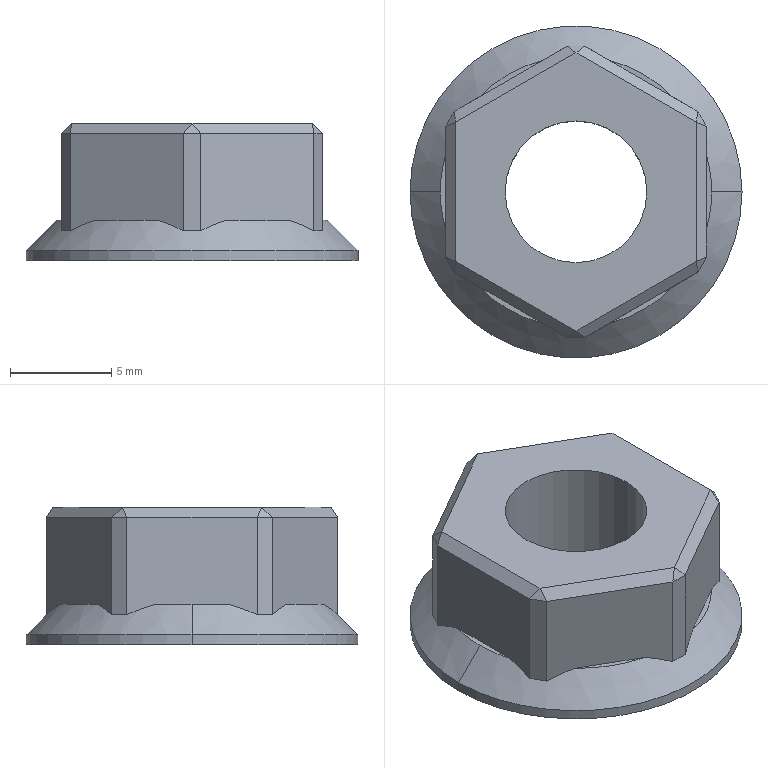Part | SolidWorks | features BaseBody 1 | 1 solid | 38 faces | box 16.4 x 16.4 x 6.8 mm | volume 790.992 mm3 | plane 32 | cylinder 4 | cone 2 | commonest cylinder face diameters 7 x2 16.4 x2
STEP:
#1=CARTESIAN_POINT('',(-8.2,0.,0.5));
#2=VERTEX_POINT('',#1);
#3=CARTESIAN_POINT('',(8.2,0.,0.5));
#4=VERTEX_POINT('',#3);
#5=CARTESIAN_POINT('',(0.,0.,0.5));
#6=DIRECTION('',(0.,0.,-1.));
#7=DIRECTION('',(-1.,0.,0.));
#8=AXIS2_PLACEMENT_3D('',#5,#6,#7);
#9=CIRCLE('',#8,8.2);
#10=EDGE_CURVE('',#2,#4,#9,.T.);
#11=ORIENTED_EDGE('',*,*,#10,.T.);
#12=CARTESIAN_POINT('',(8.2,0.,0.));
#13=VERTEX_POINT('',#12);
#14=CARTESIAN_POINT('',(8.2,0.,2.));
#15=DIRECTION('',(0.,0.,-1.));
#16=VECTOR('',#15,1000.);
#17=LINE('',#14,#16);
#18=EDGE_CURVE('',#4,#13,#17,.T.);
#19=ORIENTED_EDGE('',*,*,#18,.T.);
#20=CARTESIAN_POINT('',(-8.2,0.,0.));
#21=VERTEX_POINT('',#20);
#22=CARTESIAN_POINT('',(0.,0.,0.));
#23=DIRECTION('',(0.,0.,1.));
#24=DIRECTION('',(-1.,0.,0.));
#25=AXIS2_PLACEMENT_3D('',#22,#23,#24);
#26=CIRCLE('',#25,8.2);
#27=EDGE_CURVE('',#13,#21,#26,.T.);
#28=ORIENTED_EDGE('',*,*,#27,.T.);
#29=CARTESIAN_POINT('',(-8.2,0.,2.));
#30=DIRECTION('',(0.,0.,-1.));
#31=VECTOR('',#30,1000.);
#32=LINE('',#29,#31);
#33=EDGE_CURVE('',#2,#21,#32,.T.);
#34=ORIENTED_EDGE('',*,*,#33,.F.);
#35=EDGE_LOOP('',(#11,#19,#28,#34));
#36=FACE_OUTER_BOUND('',#35,.T.);
#37=CARTESIAN_POINT('',(0.,0.,2.));
#38=DIRECTION('',(0.,0.,-1.));
#39=DIRECTION('',(-1.,0.,0.));
#40=AXIS2_PLACEMENT_3D('',#37,#38,#39);
#41=CYLINDRICAL_SURFACE('',#40,8.2);
#42=ADVANCED_FACE('',(#36),#41,.T.);
#43=CARTESIAN_POINT('',(3.5,0.,0.));
#44=VERTEX_POINT('',#43);
#45=CARTESIAN_POINT('',(-3.5,0.,0.));
#46=VERTEX_POINT('',#45);
#47=CARTESIAN_POINT('',(0.,0.,0.));
#48=DIRECTION('',(0.,0.,-1.));
#49=DIRECTION('',(1.,0.,0.));
#50=AXIS2_PLACEMENT_3D('',#47,#48,#49);
#51=CIRCLE('',#50,3.5);
#52=EDGE_CURVE('',#44,#46,#51,.T.);
#53=ORIENTED_EDGE('',*,*,#52,.T.);
#54=CARTESIAN_POINT('',(-3.5,0.,6.8));
#55=VERTEX_POINT('',#54);
#56=CARTESIAN_POINT('',(-3.5,0.,6.8));
#57=DIRECTION('',(0.,0.,1.));
#58=VECTOR('',#57,1000.);
#59=LINE('',#56,#58);
#60=EDGE_CURVE('',#46,#55,#59,.T.);
#61=ORIENTED_EDGE('',*,*,#60,.T.);
#62=CARTESIAN_POINT('',(3.5,0.,6.8));
#63=VERTEX_POINT('',#62);
#64=CARTESIAN_POINT('',(0.,0.,6.8));
#65=DIRECTION('',(0.,0.,-1.));
#66=DIRECTION('',(1.,0.,0.));
#67=AXIS2_PLACEMENT_3D('',#64,#65,#66);
#68=CIRCLE('',#67,3.5);
#69=EDGE_CURVE('',#63,#55,#68,.T.);
#70=ORIENTED_EDGE('',*,*,#69,.F.);
#71=CARTESIAN_POINT('',(3.5,0.,6.8));
#72=DIRECTION('',(0.,0.,1.));
#73=VECTOR('',#72,1000.);
#74=LINE('',#71,#73);
#75=EDGE_CURVE('',#44,#63,#74,.T.);
#76=ORIENTED_EDGE('',*,*,#75,.F.);
#77=EDGE_LOOP('',(#53,#61,#70,#76));
#78=FACE_OUTER_BOUND('',#77,.T.);
#79=CARTESIAN_POINT('',(0.,0.,6.8));
#80=DIRECTION('',(0.,0.,1.));
#81=DIRECTION('',(1.,0.,0.));
#82=AXIS2_PLACEMENT_3D('',#79,#80,#81);
#83=CYLINDRICAL_SURFACE('',#82,3.5);
#84=ADVANCED_FACE('',(#78),#83,.F.);
#85=CARTESIAN_POINT('',(6.45,1.813,2.));
#86=VERTEX_POINT('',#85);
#87=CARTESIAN_POINT('',(6.7,0.,2.));
#88=VERTEX_POINT('',#87);
#89=CARTESIAN_POINT('',(0.,0.,2.));
#90=DIRECTION('',(0.,0.,-1.));
#91=DIRECTION('',(-1.,0.,0.));
#92=AXIS2_PLACEMENT_3D('',#89,#90,#91);
#93=CIRCLE('',#92,6.7);
#94=EDGE_CURVE('',#86,#88,#93,.T.);
#95=ORIENTED_EDGE('',*,*,#94,.T.);
#96=CARTESIAN_POINT('',(8.2,0.,0.5));
#97=DIRECTION('',(0.7071,0.,-0.7071));
#98=VECTOR('',#97,1000.);
#99=LINE('',#96,#98);
#100=EDGE_CURVE('',#88,#4,#99,.T.);
#101=ORIENTED_EDGE('',*,*,#100,.T.);
#102=ORIENTED_EDGE('',*,*,#10,.F.);
#103=CARTESIAN_POINT('',(-6.7,0.,2.));
#104=VERTEX_POINT('',#103);
#105=CARTESIAN_POINT('',(-8.2,0.,0.5));
#106=DIRECTION('',(-0.7071,0.,-0.7071));
#107=VECTOR('',#106,1000.);
#108=LINE('',#105,#107);
#109=EDGE_CURVE('',#104,#2,#108,.T.);
#110=ORIENTED_EDGE('',*,*,#109,.F.);
#111=CARTESIAN_POINT('',(-6.45,1.813,2.));
#112=VERTEX_POINT('',#111);
#113=CARTESIAN_POINT('',(0.,0.,2.));
#114=DIRECTION('',(0.,0.,-1.));
#115=DIRECTION('',(-1.,0.,0.));
#116=AXIS2_PLACEMENT_3D('',#113,#114,#115);
#117=CIRCLE('',#116,6.7);
#118=EDGE_CURVE('',#104,#112,#117,.T.);
#119=ORIENTED_EDGE('',*,*,#118,.T.);
#120=CARTESIAN_POINT('',(-6.45,3.224,1.489));
#121=VERTEX_POINT('',#120);
#122=CARTESIAN_POINT('',(-6.45,1.813,2.));
#123=CARTESIAN_POINT('',(-6.45,2.298,1.869));
#124=CARTESIAN_POINT('',(-6.45,2.766,1.694));
#125=CARTESIAN_POINT('',(-6.45,3.224,1.489));
#126=B_SPLINE_CURVE_WITH_KNOTS('',3,(#122,#123,#124,#125),.UNSPECIFIED.,.F.,.F.,(4,4),(0.,0.0015),.UNSPECIFIED.);
#127=EDGE_CURVE('',#112,#121,#126,.T.);
#128=ORIENTED_EDGE('',*,*,#127,.T.);
#129=CARTESIAN_POINT('',(-6.017,3.974,1.489));
#130=VERTEX_POINT('',#129);
#131=CARTESIAN_POINT('',(-6.45,3.224,1.489));
#132=CARTESIAN_POINT('',(-6.306,3.474,1.507));
#133=CARTESIAN_POINT('',(-6.161,3.724,1.507));
#134=CARTESIAN_POINT('',(-6.017,3.974,1.489));
#135=B_SPLINE_CURVE_WITH_KNOTS('',3,(#131,#132,#133,#134),.UNSPECIFIED.,.F.,.F.,(4,4),(0.,0.000866),.UNSPECIFIED.);
#136=EDGE_CURVE('',#121,#130,#135,.T.);
#137=ORIENTED_EDGE('',*,*,#136,.T.);
#138=CARTESIAN_POINT('',(-4.795,4.679,2.));
#139=VERTEX_POINT('',#138);
#140=CARTESIAN_POINT('',(-6.017,3.974,1.489));
#141=CARTESIAN_POINT('',(-5.621,4.203,1.694));
#142=CARTESIAN_POINT('',(-5.215,4.437,1.869));
#143=CARTESIAN_POINT('',(-4.795,4.679,2.));
#144=B_SPLINE_CURVE_WITH_KNOTS('',3,(#140,#141,#142,#143),.UNSPECIFIED.,.F.,.F.,(4,4),(0.,0.0015),.UNSPECIFIED.);
#145=EDGE_CURVE('',#130,#139,#144,.T.);
#146=ORIENTED_EDGE('',*,*,#145,.T.);
#147=CARTESIAN_POINT('',(-1.655,6.492,2.));
#148=VERTEX_POINT('',#147);
#149=CARTESIAN_POINT('',(0.,0.,2.));
#150=DIRECTION('',(0.,0.,-1.));
#151=DIRECTION('',(-1.,0.,0.));
#152=AXIS2_PLACEMENT_3D('',#149,#150,#151);
#153=CIRCLE('',#152,6.7);
#154=EDGE_CURVE('',#139,#148,#153,.T.);
#155=ORIENTED_EDGE('',*,*,#154,.T.);
#156=CARTESIAN_POINT('',(-0.433,7.198,1.489));
#157=VERTEX_POINT('',#156);
#158=CARTESIAN_POINT('',(-1.655,6.492,2.));
#159=CARTESIAN_POINT('',(-1.235,6.735,1.869));
#160=CARTESIAN_POINT('',(-0.8295,6.969,1.694));
#161=CARTESIAN_POINT('',(-0.433,7.198,1.489));
#162=B_SPLINE_CURVE_WITH_KNOTS('',3,(#158,#159,#160,#161),.UNSPECIFIED.,.F.,.F.,(4,4),(0.,0.0015),.UNSPECIFIED.);
#163=EDGE_CURVE('',#148,#157,#162,.T.);
#164=ORIENTED_EDGE('',*,*,#163,.T.);
#165=CARTESIAN_POINT('',(0.433,7.198,1.489));
#166=VERTEX_POINT('',#165);
#167=CARTESIAN_POINT('',(-0.433,7.198,1.489));
#168=CARTESIAN_POINT('',(-0.1443,7.198,1.507));
#169=CARTESIAN_POINT('',(0.1443,7.198,1.507));
#170=CARTESIAN_POINT('',(0.433,7.198,1.489));
#171=B_SPLINE_CURVE_WITH_KNOTS('',3,(#167,#168,#169,#170),.UNSPECIFIED.,.F.,.F.,(4,4),(0.,0.000866),.UNSPECIFIED.);
#172=EDGE_CURVE('',#157,#166,#171,.T.);
#173=ORIENTED_EDGE('',*,*,#172,.T.);
#174=CARTESIAN_POINT('',(1.655,6.492,2.));
#175=VERTEX_POINT('',#174);
#176=CARTESIAN_POINT('',(0.433,7.198,1.489));
#177=CARTESIAN_POINT('',(0.8295,6.969,1.694));
#178=CARTESIAN_POINT('',(1.235,6.735,1.869));
#179=CARTESIAN_POINT('',(1.655,6.492,2.));
#180=B_SPLINE_CURVE_WITH_KNOTS('',3,(#176,#177,#178,#179),.UNSPECIFIED.,.F.,.F.,(4,4),(0.,0.0015),.UNSPECIFIED.);
#181=EDGE_CURVE('',#166,#175,#180,.T.);
#182=ORIENTED_EDGE('',*,*,#181,.T.);
#183=CARTESIAN_POINT('',(4.795,4.679,2.));
#184=VERTEX_POINT('',#183);
#185=CARTESIAN_POINT('',(0.,0.,2.));
#186=DIRECTION('',(0.,0.,-1.));
#187=DIRECTION('',(-1.,0.,0.));
#188=AXIS2_PLACEMENT_3D('',#185,#186,#187);
#189=CIRCLE('',#188,6.7);
#190=EDGE_CURVE('',#175,#184,#189,.T.);
#191=ORIENTED_EDGE('',*,*,#190,.T.);
#192=CARTESIAN_POINT('',(6.017,3.974,1.489));
#193=VERTEX_POINT('',#192);
#194=CARTESIAN_POINT('',(4.795,4.679,2.));
#195=CARTESIAN_POINT('',(5.215,4.437,1.869));
#196=CARTESIAN_POINT('',(5.621,4.203,1.694));
#197=CARTESIAN_POINT('',(6.017,3.974,1.489));
#198=B_SPLINE_CURVE_WITH_KNOTS('',3,(#194,#195,#196,#197),.UNSPECIFIED.,.F.,.F.,(4,4),(0.,0.0015),.UNSPECIFIED.);
#199=EDGE_CURVE('',#184,#193,#198,.T.);
#200=ORIENTED_EDGE('',*,*,#199,.T.);
#201=CARTESIAN_POINT('',(6.45,3.224,1.489));
#202=VERTEX_POINT('',#201);
#203=CARTESIAN_POINT('',(6.017,3.974,1.489));
#204=CARTESIAN_POINT('',(6.161,3.724,1.507));
#205=CARTESIAN_POINT('',(6.306,3.474,1.507));
#206=CARTESIAN_POINT('',(6.45,3.224,1.489));
#207=B_SPLINE_CURVE_WITH_KNOTS('',3,(#203,#204,#205,#206),.UNSPECIFIED.,.F.,.F.,(4,4),(0.,0.000866),.UNSPECIFIED.);
#208=EDGE_CURVE('',#193,#202,#207,.T.);
#209=ORIENTED_EDGE('',*,*,#208,.T.);
#210=CARTESIAN_POINT('',(6.45,3.224,1.489));
#211=CARTESIAN_POINT('',(6.45,2.766,1.694));
#212=CARTESIAN_POINT('',(6.45,2.298,1.869));
#213=CARTESIAN_POINT('',(6.45,1.813,2.));
#214=B_SPLINE_CURVE_WITH_KNOTS('',3,(#210,#211,#212,#213),.UNSPECIFIED.,.F.,.F.,(4,4),(0.,0.0015),.UNSPECIFIED.);
#215=EDGE_CURVE('',#202,#86,#214,.T.);
#216=ORIENTED_EDGE('',*,*,#215,.T.);
#217=EDGE_LOOP('',(#95,#101,#102,#110,#119,#128,#137,#146,#155,#164,#173,#182,#191,#200,#209,#216));
#218=FACE_OUTER_BOUND('',#217,.T.);
#219=CARTESIAN_POINT('',(0.,0.,0.5));
#220=DIRECTION('',(0.,0.,-1.));
#221=DIRECTION('',(-1.,0.,0.));
#222=AXIS2_PLACEMENT_3D('',#219,#220,#221);
#223=CONICAL_SURFACE('',#222,8.2,0.7854);
#224=ADVANCED_FACE('',(#218),#223,.T.);
#225=CARTESIAN_POINT('',(0.,0.,0.));
#226=DIRECTION('',(0.,0.,1.));
#227=DIRECTION('',(-1.,0.,0.));
#228=AXIS2_PLACEMENT_3D('',#225,#226,#227);
#229=CIRCLE('',#228,8.2);
#230=EDGE_CURVE('',#21,#13,#229,.T.);
#231=ORIENTED_EDGE('',*,*,#230,.F.);
#232=ORIENTED_EDGE('',*,*,#27,.F.);
#233=EDGE_LOOP('',(#231,#232));
#234=FACE_OUTER_BOUND('',#233,.T.);
#235=ORIENTED_EDGE('',*,*,#52,.F.);
#236=CARTESIAN_POINT('',(0.,0.,0.));
#237=DIRECTION('',(0.,0.,-1.));
#238=DIRECTION('',(1.,0.,0.));
#239=AXIS2_PLACEMENT_3D('',#236,#237,#238);
#240=CIRCLE('',#239,3.5);
#241=EDGE_CURVE('',#46,#44,#240,.T.);
#242=ORIENTED_EDGE('',*,*,#241,.F.);
#243=EDGE_LOOP('',(#235,#242));
#244=FACE_BOUND('',#243,.T.);
#245=CARTESIAN_POINT('',(0.,0.,0.));
#246=DIRECTION('',(0.,0.,1.));
#247=DIRECTION('',(1.,0.,0.));
#248=AXIS2_PLACEMENT_3D('',#245,#246,#247);
#249=PLANE('',#248);
#250=ADVANCED_FACE('',(#234,#244),#249,.F.);
#251=ORIENTED_EDGE('',*,*,#18,.F.);
#252=CARTESIAN_POINT('',(0.,0.,0.5));
#253=DIRECTION('',(0.,0.,-1.));
#254=DIRECTION('',(-1.,0.,0.));
#255=AXIS2_PLACEMENT_3D('',#252,#253,#254);
#256=CIRCLE('',#255,8.2);
#257=EDGE_CURVE('',#4,#2,#256,.T.);
#258=ORIENTED_EDGE('',*,*,#257,.T.);
#259=ORIENTED_EDGE('',*,*,#33,.T.);
#260=ORIENTED_EDGE('',*,*,#230,.T.);
#261=EDGE_LOOP('',(#251,#258,#259,#260));
#262=FACE_OUTER_BOUND('',#261,.T.);
#263=CARTESIAN_POINT('',(0.,0.,2.));
#264=DIRECTION('',(0.,0.,-1.));
#265=DIRECTION('',(-1.,0.,0.));
#266=AXIS2_PLACEMENT_3D('',#263,#264,#265);
#267=CYLINDRICAL_SURFACE('',#266,8.2);
#268=ADVANCED_FACE('',(#262),#267,.T.);
#269=ORIENTED_EDGE('',*,*,#60,.F.);
#270=ORIENTED_EDGE('',*,*,#241,.T.);
#271=ORIENTED_EDGE('',*,*,#75,.T.);
#272=CARTESIAN_POINT('',(0.,0.,6.8));
#273=DIRECTION('',(0.,0.,-1.));
#274=DIRECTION('',(1.,0.,0.));
#275=AXIS2_PLACEMENT_3D('',#272,#273,#274);
#276=CIRCLE('',#275,3.5);
#277=EDGE_CURVE('',#55,#63,#276,.T.);
#278=ORIENTED_EDGE('',*,*,#277,.F.);
#279=EDGE_LOOP('',(#269,#270,#271,#278));
#280=FACE_OUTER_BOUND('',#279,.T.);
#281=CARTESIAN_POINT('',(0.,0.,6.8));
#282=DIRECTION('',(0.,0.,1.));
#283=DIRECTION('',(1.,0.,0.));
#284=AXIS2_PLACEMENT_3D('',#281,#282,#283);
#285=CYLINDRICAL_SURFACE('',#284,3.5);
#286=ADVANCED_FACE('',(#280),#285,.F.);
#287=ORIENTED_EDGE('',*,*,#100,.F.);
#288=CARTESIAN_POINT('',(6.45,-1.813,2.));
#289=VERTEX_POINT('',#288);
#290=CARTESIAN_POINT('',(0.,0.,2.));
#291=DIRECTION('',(0.,0.,-1.));
#292=DIRECTION('',(-1.,0.,0.));
#293=AXIS2_PLACEMENT_3D('',#290,#291,#292);
#294=CIRCLE('',#293,6.7);
#295=EDGE_CURVE('',#88,#289,#294,.T.);
#296=ORIENTED_EDGE('',*,*,#295,.T.);
#297=CARTESIAN_POINT('',(6.45,-3.224,1.489));
#298=VERTEX_POINT('',#297);
#299=CARTESIAN_POINT('',(6.45,-1.813,2.));
#300=CARTESIAN_POINT('',(6.45,-2.298,1.869));
#301=CARTESIAN_POINT('',(6.45,-2.766,1.694));
#302=CARTESIAN_POINT('',(6.45,-3.224,1.489));
#303=B_SPLINE_CURVE_WITH_KNOTS('',3,(#299,#300,#301,#302),.UNSPECIFIED.,.F.,.F.,(4,4),(0.,0.0015),.UNSPECIFIED.);
#304=EDGE_CURVE('',#289,#298,#303,.T.);
#305=ORIENTED_EDGE('',*,*,#304,.T.);
#306=CARTESIAN_POINT('',(6.017,-3.974,1.489));
#307=VERTEX_POINT('',#306);
#308=CARTESIAN_POINT('',(6.45,-3.224,1.489));
#309=CARTESIAN_POINT('',(6.306,-3.474,1.507));
#310=CARTESIAN_POINT('',(6.161,-3.724,1.507));
#311=CARTESIAN_POINT('',(6.017,-3.974,1.489));
#312=B_SPLINE_CURVE_WITH_KNOTS('',3,(#308,#309,#310,#311),.UNSPECIFIED.,.F.,.F.,(4,4),(0.,0.000866),.UNSPECIFIED.);
#313=EDGE_CURVE('',#298,#307,#312,.T.);
#314=ORIENTED_EDGE('',*,*,#313,.T.);
#315=CARTESIAN_POINT('',(4.795,-4.679,2.));
#316=VERTEX_POINT('',#315);
#317=CARTESIAN_POINT('',(6.017,-3.974,1.489));
#318=CARTESIAN_POINT('',(5.621,-4.203,1.694));
#319=CARTESIAN_POINT('',(5.215,-4.437,1.869));
#320=CARTESIAN_POINT('',(4.795,-4.679,2.));
#321=B_SPLINE_CURVE_WITH_KNOTS('',3,(#317,#318,#319,#320),.UNSPECIFIED.,.F.,.F.,(4,4),(0.,0.0015),.UNSPECIFIED.);
#322=EDGE_CURVE('',#307,#316,#321,.T.);
#323=ORIENTED_EDGE('',*,*,#322,.T.);
#324=CARTESIAN_POINT('',(1.655,-6.492,2.));
#325=VERTEX_POINT('',#324);
#326=CARTESIAN_POINT('',(0.,0.,2.));
#327=DIRECTION('',(0.,0.,-1.));
#328=DIRECTION('',(-1.,0.,0.));
#329=AXIS2_PLACEMENT_3D('',#326,#327,#328);
#330=CIRCLE('',#329,6.7);
#331=EDGE_CURVE('',#316,#325,#330,.T.);
#332=ORIENTED_EDGE('',*,*,#331,.T.);
#333=CARTESIAN_POINT('',(0.433,-7.198,1.489));
#334=VERTEX_POINT('',#333);
#335=CARTESIAN_POINT('',(1.655,-6.492,2.));
#336=CARTESIAN_POINT('',(1.235,-6.735,1.869));
#337=CARTESIAN_POINT('',(0.8295,-6.969,1.694));
#338=CARTESIAN_POINT('',(0.433,-7.198,1.489));
#339=B_SPLINE_CURVE_WITH_KNOTS('',3,(#335,#336,#337,#338),.UNSPECIFIED.,.F.,.F.,(4,4),(0.,0.0015),.UNSPECIFIED.);
#340=EDGE_CURVE('',#325,#334,#339,.T.);
#341=ORIENTED_EDGE('',*,*,#340,.T.);
#342=CARTESIAN_POINT('',(-0.433,-7.198,1.489));
#343=VERTEX_POINT('',#342);
#344=CARTESIAN_POINT('',(0.433,-7.198,1.489));
#345=CARTESIAN_POINT('',(0.1443,-7.198,1.507));
#346=CARTESIAN_POINT('',(-0.1443,-7.198,1.507));
#347=CARTESIAN_POINT('',(-0.433,-7.198,1.489));
#348=B_SPLINE_CURVE_WITH_KNOTS('',3,(#344,#345,#346,#347),.UNSPECIFIED.,.F.,.F.,(4,4),(0.,0.000866),.UNSPECIFIED.);
#349=EDGE_CURVE('',#334,#343,#348,.T.);
#350=ORIENTED_EDGE('',*,*,#349,.T.);
#351=CARTESIAN_POINT('',(-1.655,-6.492,2.));
#352=VERTEX_POINT('',#351);
#353=CARTESIAN_POINT('',(-0.433,-7.198,1.489));
#354=CARTESIAN_POINT('',(-0.8295,-6.969,1.694));
#355=CARTESIAN_POINT('',(-1.235,-6.735,1.869));
#356=CARTESIAN_POINT('',(-1.655,-6.492,2.));
#357=B_SPLINE_CURVE_WITH_KNOTS('',3,(#353,#354,#355,#356),.UNSPECIFIED.,.F.,.F.,(4,4),(0.,0.0015),.UNSPECIFIED.);
#358=EDGE_CURVE('',#343,#352,#357,.T.);
#359=ORIENTED_EDGE('',*,*,#358,.T.);
#360=CARTESIAN_POINT('',(-4.795,-4.679,2.));
#361=VERTEX_POINT('',#360);
#362=CARTESIAN_POINT('',(0.,0.,2.));
#363=DIRECTION('',(0.,0.,-1.));
#364=DIRECTION('',(-1.,0.,0.));
#365=AXIS2_PLACEMENT_3D('',#362,#363,#364);
#366=CIRCLE('',#365,6.7);
#367=EDGE_CURVE('',#352,#361,#366,.T.);
#368=ORIENTED_EDGE('',*,*,#367,.T.);
#369=CARTESIAN_POINT('',(-6.017,-3.974,1.489));
#370=VERTEX_POINT('',#369);
#371=CARTESIAN_POINT('',(-4.795,-4.679,2.));
#372=CARTESIAN_POINT('',(-5.215,-4.437,1.869));
#373=CARTESIAN_POINT('',(-5.621,-4.203,1.694));
#374=CARTESIAN_POINT('',(-6.017,-3.974,1.489));
#375=B_SPLINE_CURVE_WITH_KNOTS('',3,(#371,#372,#373,#374),.UNSPECIFIED.,.F.,.F.,(4,4),(0.,0.0015),.UNSPECIFIED.);
#376=EDGE_CURVE('',#361,#370,#375,.T.);
#377=ORIENTED_EDGE('',*,*,#376,.T.);
#378=CARTESIAN_POINT('',(-6.45,-3.224,1.489));
#379=VERTEX_POINT('',#378);
#380=CARTESIAN_POINT('',(-6.017,-3.974,1.489));
#381=CARTESIAN_POINT('',(-6.161,-3.724,1.507));
#382=CARTESIAN_POINT('',(-6.306,-3.474,1.507));
#383=CARTESIAN_POINT('',(-6.45,-3.224,1.489));
#384=B_SPLINE_CURVE_WITH_KNOTS('',3,(#380,#381,#382,#383),.UNSPECIFIED.,.F.,.F.,(4,4),(0.,0.000866),.UNSPECIFIED.);
#385=EDGE_CURVE('',#370,#379,#384,.T.);
#386=ORIENTED_EDGE('',*,*,#385,.T.);
#387=CARTESIAN_POINT('',(-6.45,-1.813,2.));
#388=VERTEX_POINT('',#387);
#389=CARTESIAN_POINT('',(-6.45,-3.224,1.489));
#390=CARTESIAN_POINT('',(-6.45,-2.766,1.694));
#391=CARTESIAN_POINT('',(-6.45,-2.298,1.869));
#392=CARTESIAN_POINT('',(-6.45,-1.813,2.));
#393=B_SPLINE_CURVE_WITH_KNOTS('',3,(#389,#390,#391,#392),.UNSPECIFIED.,.F.,.F.,(4,4),(0.,0.0015),.UNSPECIFIED.);
#394=EDGE_CURVE('',#379,#388,#393,.T.);
#395=ORIENTED_EDGE('',*,*,#394,.T.);
#396=CARTESIAN_POINT('',(0.,0.,2.));
#397=DIRECTION('',(0.,0.,-1.));
#398=DIRECTION('',(-1.,0.,0.));
#399=AXIS2_PLACEMENT_3D('',#396,#397,#398);
#400=CIRCLE('',#399,6.7);
#401=EDGE_CURVE('',#388,#104,#400,.T.);
#402=ORIENTED_EDGE('',*,*,#401,.T.);
#403=ORIENTED_EDGE('',*,*,#109,.T.);
#404=ORIENTED_EDGE('',*,*,#257,.F.);
#405=EDGE_LOOP('',(#287,#296,#305,#314,#323,#332,#341,#350,#359,#368,#377,#386,#395,#402,#403,#404));
#406=FACE_OUTER_BOUND('',#405,.T.);
#407=CARTESIAN_POINT('',(0.,0.,0.5));
#408=DIRECTION('',(0.,0.,-1.));
#409=DIRECTION('',(-1.,0.,0.));
#410=AXIS2_PLACEMENT_3D('',#407,#408,#409);
#411=CONICAL_SURFACE('',#410,8.2,0.7854);
#412=ADVANCED_FACE('',(#406),#411,.T.);
#413=ORIENTED_EDGE('',*,*,#69,.T.);
#414=ORIENTED_EDGE('',*,*,#277,.T.);
#415=EDGE_LOOP('',(#413,#414));
#416=FACE_BOUND('',#415,.T.);
#417=CARTESIAN_POINT('',(-5.95,3.435,6.8));
#418=VERTEX_POINT('',#417);
#419=CARTESIAN_POINT('',(-5.95,-3.435,6.8));
#420=VERTEX_POINT('',#419);
#421=CARTESIAN_POINT('',(-5.95,0.,6.8));
#422=DIRECTION('',(0.,-1.,0.));
#423=VECTOR('',#422,1000.);
#424=LINE('',#421,#423);
#425=EDGE_CURVE('',#418,#420,#424,.T.);
#426=ORIENTED_EDGE('',*,*,#425,.T.);
#427=CARTESIAN_POINT('',(0.,-6.87,6.8));
#428=VERTEX_POINT('',#427);
#429=CARTESIAN_POINT('',(-5.95,-3.435,6.8));
#430=DIRECTION('',(0.866,-0.5,0.));
#431=VECTOR('',#430,1000.);
#432=LINE('',#429,#431);
#433=EDGE_CURVE('',#420,#428,#432,.T.);
#434=ORIENTED_EDGE('',*,*,#433,.T.);
#435=CARTESIAN_POINT('',(5.95,-3.435,6.8));
#436=VERTEX_POINT('',#435);
#437=CARTESIAN_POINT('',(0.,-6.87,6.8));
#438=DIRECTION('',(0.866,0.5,0.));
#439=VECTOR('',#438,1000.);
#440=LINE('',#437,#439);
#441=EDGE_CURVE('',#428,#436,#440,.T.);
#442=ORIENTED_EDGE('',*,*,#441,.T.);
#443=CARTESIAN_POINT('',(5.95,3.435,6.8));
#444=VERTEX_POINT('',#443);
#445=CARTESIAN_POINT('',(5.95,0.,6.8));
#446=DIRECTION('',(0.,1.,0.));
#447=VECTOR('',#446,1000.);
#448=LINE('',#445,#447);
#449=EDGE_CURVE('',#436,#444,#448,.T.);
#450=ORIENTED_EDGE('',*,*,#449,.T.);
#451=CARTESIAN_POINT('',(0.,6.87,6.8));
#452=VERTEX_POINT('',#451);
#453=CARTESIAN_POINT('',(5.95,3.435,6.8));
#454=DIRECTION('',(-0.866,0.5,0.));
#455=VECTOR('',#454,1000.);
#456=LINE('',#453,#455);
#457=EDGE_CURVE('',#444,#452,#456,.T.);
#458=ORIENTED_EDGE('',*,*,#457,.T.);
#459=CARTESIAN_POINT('',(0.,6.87,6.8));
#460=DIRECTION('',(-0.866,-0.5,0.));
#461=VECTOR('',#460,1000.);
#462=LINE('',#459,#461);
#463=EDGE_CURVE('',#452,#418,#462,.T.);
#464=ORIENTED_EDGE('',*,*,#463,.T.);
#465=EDGE_LOOP('',(#426,#434,#442,#450,#458,#464));
#466=FACE_OUTER_BOUND('',#465,.T.);
#467=CARTESIAN_POINT('',(0.,0.,6.8));
#468=DIRECTION('',(0.,0.,1.));
#469=DIRECTION('',(1.,0.,0.));
#470=AXIS2_PLACEMENT_3D('',#467,#468,#469);
#471=PLANE('',#470);
#472=ADVANCED_FACE('',(#416,#466),#471,.T.);
#473=ORIENTED_EDGE('',*,*,#190,.F.);
#474=CARTESIAN_POINT('',(4.795,4.679,2.));
#475=DIRECTION('',(-0.866,0.5,0.));
#476=VECTOR('',#475,1000.);
#477=LINE('',#474,#476);
#478=EDGE_CURVE('',#184,#175,#477,.T.);
#479=ORIENTED_EDGE('',*,*,#478,.F.);
#480=EDGE_LOOP('',(#473,#479));
#481=FACE_OUTER_BOUND('',#480,.T.);
#482=CARTESIAN_POINT('',(0.,0.,2.));
#483=DIRECTION('',(0.,0.,-1.));
#484=DIRECTION('',(-1.,0.,0.));
#485=AXIS2_PLACEMENT_3D('',#482,#483,#484);
#486=PLANE('',#485);
#487=ADVANCED_FACE('',(#481),#486,.F.);
#488=ORIENTED_EDGE('',*,*,#154,.F.);
#489=CARTESIAN_POINT('',(-1.655,6.492,2.));
#490=DIRECTION('',(-0.866,-0.5,0.));
#491=VECTOR('',#490,1000.);
#492=LINE('',#489,#491);
#493=EDGE_CURVE('',#148,#139,#492,.T.);
#494=ORIENTED_EDGE('',*,*,#493,.F.);
#495=EDGE_LOOP('',(#488,#494));
#496=FACE_OUTER_BOUND('',#495,.T.);
#497=CARTESIAN_POINT('',(0.,0.,2.));
#498=DIRECTION('',(0.,0.,-1.));
#499=DIRECTION('',(-1.,0.,0.));
#500=AXIS2_PLACEMENT_3D('',#497,#498,#499);
#501=PLANE('',#500);
#502=ADVANCED_FACE('',(#496),#501,.F.);
#503=ORIENTED_EDGE('',*,*,#401,.F.);
#504=CARTESIAN_POINT('',(-6.45,0.,2.));
#505=DIRECTION('',(0.,-1.,0.));
#506=VECTOR('',#505,1000.);
#507=LINE('',#504,#506);
#508=EDGE_CURVE('',#112,#388,#507,.T.);
#509=ORIENTED_EDGE('',*,*,#508,.F.);
#510=ORIENTED_EDGE('',*,*,#118,.F.);
#511=EDGE_LOOP('',(#503,#509,#510));
#512=FACE_OUTER_BOUND('',#511,.T.);
#513=CARTESIAN_POINT('',(0.,0.,2.));
#514=DIRECTION('',(0.,0.,-1.));
#515=DIRECTION('',(-1.,0.,0.));
#516=AXIS2_PLACEMENT_3D('',#513,#514,#515);
#517=PLANE('',#516);
#518=ADVANCED_FACE('',(#512),#517,.F.);
#519=CARTESIAN_POINT('',(6.45,0.,2.));
#520=DIRECTION('',(0.,1.,0.));
#521=VECTOR('',#520,1000.);
#522=LINE('',#519,#521);
#523=EDGE_CURVE('',#289,#86,#522,.T.);
#524=ORIENTED_EDGE('',*,*,#523,.F.);
#525=ORIENTED_EDGE('',*,*,#295,.F.);
#526=ORIENTED_EDGE('',*,*,#94,.F.);
#527=EDGE_LOOP('',(#524,#525,#526));
#528=FACE_OUTER_BOUND('',#527,.T.);
#529=CARTESIAN_POINT('',(0.,0.,2.));
#530=DIRECTION('',(0.,0.,-1.));
#531=DIRECTION('',(-1.,0.,0.));
#532=AXIS2_PLACEMENT_3D('',#529,#530,#531);
#533=PLANE('',#532);
#534=ADVANCED_FACE('',(#528),#533,.F.);
#535=ORIENTED_EDGE('',*,*,#367,.F.);
#536=CARTESIAN_POINT('',(-4.795,-4.679,2.));
#537=DIRECTION('',(0.866,-0.5,0.));
#538=VECTOR('',#537,1000.);
#539=LINE('',#536,#538);
#540=EDGE_CURVE('',#361,#352,#539,.T.);
#541=ORIENTED_EDGE('',*,*,#540,.F.);
#542=EDGE_LOOP('',(#535,#541));
#543=FACE_OUTER_BOUND('',#542,.T.);
#544=CARTESIAN_POINT('',(0.,0.,2.));
#545=DIRECTION('',(0.,0.,-1.));
#546=DIRECTION('',(-1.,0.,0.));
#547=AXIS2_PLACEMENT_3D('',#544,#545,#546);
#548=PLANE('',#547);
#549=ADVANCED_FACE('',(#543),#548,.F.);
#550=ORIENTED_EDGE('',*,*,#331,.F.);
#551=CARTESIAN_POINT('',(1.655,-6.492,2.));
#552=DIRECTION('',(0.866,0.5,0.));
#553=VECTOR('',#552,1000.);
#554=LINE('',#551,#553);
#555=EDGE_CURVE('',#325,#316,#554,.T.);
#556=ORIENTED_EDGE('',*,*,#555,.F.);
#557=EDGE_LOOP('',(#550,#556));
#558=FACE_OUTER_BOUND('',#557,.T.);
#559=CARTESIAN_POINT('',(0.,0.,2.));
#560=DIRECTION('',(0.,0.,-1.));
#561=DIRECTION('',(-1.,0.,0.));
#562=AXIS2_PLACEMENT_3D('',#559,#560,#561);
#563=PLANE('',#562);
#564=ADVANCED_FACE('',(#558),#563,.F.);
#565=CARTESIAN_POINT('',(-0.433,-7.198,6.3));
#566=VERTEX_POINT('',#565);
#567=CARTESIAN_POINT('',(-0.433,-7.198,6.3));
#568=DIRECTION('',(0.5867,0.4436,0.6775));
#569=VECTOR('',#568,1000.);
#570=LINE('',#567,#569);
#571=EDGE_CURVE('',#566,#428,#570,.T.);
#572=ORIENTED_EDGE('',*,*,#571,.T.);
#573=ORIENTED_EDGE('',*,*,#433,.F.);
#574=CARTESIAN_POINT('',(-6.017,-3.974,6.3));
#575=VERTEX_POINT('',#574);
#576=CARTESIAN_POINT('',(-5.95,-3.435,6.8));
#577=DIRECTION('',(-0.09077,-0.7299,-0.6775));
#578=VECTOR('',#577,1000.);
#579=LINE('',#576,#578);
#580=EDGE_CURVE('',#420,#575,#579,.T.);
#581=ORIENTED_EDGE('',*,*,#580,.T.);
#582=CARTESIAN_POINT('',(-6.017,-3.974,6.3));
#583=DIRECTION('',(0.866,-0.5,0.));
#584=VECTOR('',#583,1000.);
#585=LINE('',#582,#584);
#586=EDGE_CURVE('',#575,#566,#585,.T.);
#587=ORIENTED_EDGE('',*,*,#586,.T.);
#588=EDGE_LOOP('',(#572,#573,#581,#587));
#589=FACE_OUTER_BOUND('',#588,.T.);
#590=CARTESIAN_POINT('',(-2.975,-5.153,6.8));
#591=DIRECTION('',(-0.3536,-0.6124,0.7071));
#592=DIRECTION('',(0.,-0.7559,-0.6547));
#593=AXIS2_PLACEMENT_3D('',#590,#591,#592);
#594=PLANE('',#593);
#595=ADVANCED_FACE('',(#589),#594,.T.);
#596=CARTESIAN_POINT('',(-6.45,-3.224,6.3));
#597=VERTEX_POINT('',#596);
#598=CARTESIAN_POINT('',(-6.45,-3.224,6.3));
#599=DIRECTION('',(0.6775,-0.2863,0.6775));
#600=VECTOR('',#599,1000.);
#601=LINE('',#598,#600);
#602=EDGE_CURVE('',#597,#420,#601,.T.);
#603=ORIENTED_EDGE('',*,*,#602,.T.);
#604=ORIENTED_EDGE('',*,*,#425,.F.);
#605=CARTESIAN_POINT('',(-6.45,3.224,6.3));
#606=VERTEX_POINT('',#605);
#607=CARTESIAN_POINT('',(-5.95,3.435,6.8));
#608=DIRECTION('',(-0.6775,-0.2863,-0.6775));
#609=VECTOR('',#608,1000.);
#610=LINE('',#607,#609);
#611=EDGE_CURVE('',#418,#606,#610,.T.);
#612=ORIENTED_EDGE('',*,*,#611,.T.);
#613=CARTESIAN_POINT('',(-6.45,0.,6.3));
#614=DIRECTION('',(0.,-1.,0.));
#615=VECTOR('',#614,1000.);
#616=LINE('',#613,#615);
#617=EDGE_CURVE('',#606,#597,#616,.T.);
#618=ORIENTED_EDGE('',*,*,#617,.T.);
#619=EDGE_LOOP('',(#603,#604,#612,#618));
#620=FACE_OUTER_BOUND('',#619,.T.);
#621=CARTESIAN_POINT('',(-5.95,0.,6.8));
#622=DIRECTION('',(-0.7071,0.,0.7071));
#623=DIRECTION('',(0.7071,0.,0.7071));
#624=AXIS2_PLACEMENT_3D('',#621,#622,#623);
#625=PLANE('',#624);
#626=ADVANCED_FACE('',(#620),#625,.T.);
#627=CARTESIAN_POINT('',(-0.433,7.198,6.3));
#628=VERTEX_POINT('',#627);
#629=CARTESIAN_POINT('',(0.,6.87,6.8));
#630=DIRECTION('',(-0.5867,0.4436,-0.6775));
#631=VECTOR('',#630,1000.);
#632=LINE('',#629,#631);
#633=EDGE_CURVE('',#452,#628,#632,.T.);
#634=ORIENTED_EDGE('',*,*,#633,.T.);
#635=CARTESIAN_POINT('',(-6.017,3.974,6.3));
#636=VERTEX_POINT('',#635);
#637=CARTESIAN_POINT('',(-0.433,7.198,6.3));
#638=DIRECTION('',(-0.866,-0.5,0.));
#639=VECTOR('',#638,1000.);
#640=LINE('',#637,#639);
#641=EDGE_CURVE('',#628,#636,#640,.T.);
#642=ORIENTED_EDGE('',*,*,#641,.T.);
#643=CARTESIAN_POINT('',(-6.017,3.974,6.3));
#644=DIRECTION('',(0.09077,-0.7299,0.6775));
#645=VECTOR('',#644,1000.);
#646=LINE('',#643,#645);
#647=EDGE_CURVE('',#636,#418,#646,.T.);
#648=ORIENTED_EDGE('',*,*,#647,.T.);
#649=ORIENTED_EDGE('',*,*,#463,.F.);
#650=EDGE_LOOP('',(#634,#642,#648,#649));
#651=FACE_OUTER_BOUND('',#650,.T.);
#652=CARTESIAN_POINT('',(-2.975,5.153,6.8));
#653=DIRECTION('',(-0.3536,0.6124,0.7071));
#654=DIRECTION('',(0.,-0.7559,0.6547));
#655=AXIS2_PLACEMENT_3D('',#652,#653,#654);
#656=PLANE('',#655);
#657=ADVANCED_FACE('',(#651),#656,.T.);
#658=CARTESIAN_POINT('',(6.017,3.974,6.3));
#659=VERTEX_POINT('',#658);
#660=CARTESIAN_POINT('',(5.95,3.435,6.8));
#661=DIRECTION('',(0.09077,0.7299,-0.6775));
#662=VECTOR('',#661,1000.);
#663=LINE('',#660,#662);
#664=EDGE_CURVE('',#444,#659,#663,.T.);
#665=ORIENTED_EDGE('',*,*,#664,.T.);
#666=CARTESIAN_POINT('',(0.433,7.198,6.3));
#667=VERTEX_POINT('',#666);
#668=CARTESIAN_POINT('',(6.017,3.974,6.3));
#669=DIRECTION('',(-0.866,0.5,0.));
#670=VECTOR('',#669,1000.);
#671=LINE('',#668,#670);
#672=EDGE_CURVE('',#659,#667,#671,.T.);
#673=ORIENTED_EDGE('',*,*,#672,.T.);
#674=CARTESIAN_POINT('',(0.433,7.198,6.3));
#675=DIRECTION('',(-0.5867,-0.4436,0.6775));
#676=VECTOR('',#675,1000.);
#677=LINE('',#674,#676);
#678=EDGE_CURVE('',#667,#452,#677,.T.);
#679=ORIENTED_EDGE('',*,*,#678,.T.);
#680=ORIENTED_EDGE('',*,*,#457,.F.);
#681=EDGE_LOOP('',(#665,#673,#679,#680));
#682=FACE_OUTER_BOUND('',#681,.T.);
#683=CARTESIAN_POINT('',(2.975,5.153,6.8));
#684=DIRECTION('',(0.3536,0.6124,0.7071));
#685=DIRECTION('',(0.,-0.7559,0.6547));
#686=AXIS2_PLACEMENT_3D('',#683,#684,#685);
#687=PLANE('',#686);
#688=ADVANCED_FACE('',(#682),#687,.T.);
#689=CARTESIAN_POINT('',(6.45,3.224,6.3));
#690=VERTEX_POINT('',#689);
#691=CARTESIAN_POINT('',(6.45,3.224,6.3));
#692=DIRECTION('',(-0.6775,0.2863,0.6775));
#693=VECTOR('',#692,1000.);
#694=LINE('',#691,#693);
#695=EDGE_CURVE('',#690,#444,#694,.T.);
#696=ORIENTED_EDGE('',*,*,#695,.T.);
#697=ORIENTED_EDGE('',*,*,#449,.F.);
#698=CARTESIAN_POINT('',(6.45,-3.224,6.3));
#699=VERTEX_POINT('',#698);
#700=CARTESIAN_POINT('',(5.95,-3.435,6.8));
#701=DIRECTION('',(0.6775,0.2863,-0.6775));
#702=VECTOR('',#701,1000.);
#703=LINE('',#700,#702);
#704=EDGE_CURVE('',#436,#699,#703,.T.);
#705=ORIENTED_EDGE('',*,*,#704,.T.);
#706=CARTESIAN_POINT('',(6.45,0.,6.3));
#707=DIRECTION('',(0.,1.,0.));
#708=VECTOR('',#707,1000.);
#709=LINE('',#706,#708);
#710=EDGE_CURVE('',#699,#690,#709,.T.);
#711=ORIENTED_EDGE('',*,*,#710,.T.);
#712=EDGE_LOOP('',(#696,#697,#705,#711));
#713=FACE_OUTER_BOUND('',#712,.T.);
#714=CARTESIAN_POINT('',(5.95,0.,6.8));
#715=DIRECTION('',(0.7071,0.,0.7071));
#716=DIRECTION('',(0.7071,0.,-0.7071));
#717=AXIS2_PLACEMENT_3D('',#714,#715,#716);
#718=PLANE('',#717);
#719=ADVANCED_FACE('',(#713),#718,.T.);
#720=CARTESIAN_POINT('',(6.017,-3.974,6.3));
#721=VERTEX_POINT('',#720);
#722=CARTESIAN_POINT('',(6.017,-3.974,6.3));
#723=DIRECTION('',(-0.09077,0.7299,0.6775));
#724=VECTOR('',#723,1000.);
#725=LINE('',#722,#724);
#726=EDGE_CURVE('',#721,#436,#725,.T.);
#727=ORIENTED_EDGE('',*,*,#726,.T.);
#728=ORIENTED_EDGE('',*,*,#441,.F.);
#729=CARTESIAN_POINT('',(0.433,-7.198,6.3));
#730=VERTEX_POINT('',#729);
#731=CARTESIAN_POINT('',(0.,-6.87,6.8));
#732=DIRECTION('',(0.5867,-0.4436,-0.6775));
#733=VECTOR('',#732,1000.);
#734=LINE('',#731,#733);
#735=EDGE_CURVE('',#428,#730,#734,.T.);
#736=ORIENTED_EDGE('',*,*,#735,.T.);
#737=CARTESIAN_POINT('',(0.433,-7.198,6.3));
#738=DIRECTION('',(0.866,0.5,0.));
#739=VECTOR('',#738,1000.);
#740=LINE('',#737,#739);
#741=EDGE_CURVE('',#730,#721,#740,.T.);
#742=ORIENTED_EDGE('',*,*,#741,.T.);
#743=EDGE_LOOP('',(#727,#728,#736,#742));
#744=FACE_OUTER_BOUND('',#743,.T.);
#745=CARTESIAN_POINT('',(2.975,-5.153,6.8));
#746=DIRECTION('',(0.3536,-0.6124,0.7071));
#747=DIRECTION('',(0.,-0.7559,-0.6547));
#748=AXIS2_PLACEMENT_3D('',#745,#746,#747);
#749=PLANE('',#748);
#750=ADVANCED_FACE('',(#744),#749,.T.);
#751=CARTESIAN_POINT('',(6.017,3.974,6.8));
#752=DIRECTION('',(0.,0.,1.));
#753=VECTOR('',#752,1000.);
#754=LINE('',#751,#753);
#755=EDGE_CURVE('',#193,#659,#754,.T.);
#756=ORIENTED_EDGE('',*,*,#755,.F.);
#757=ORIENTED_EDGE('',*,*,#199,.F.);
#758=ORIENTED_EDGE('',*,*,#478,.T.);
#759=ORIENTED_EDGE('',*,*,#181,.F.);
#760=CARTESIAN_POINT('',(0.433,7.198,6.8));
#761=DIRECTION('',(0.,0.,-1.));
#762=VECTOR('',#761,1000.);
#763=LINE('',#760,#762);
#764=EDGE_CURVE('',#667,#166,#763,.T.);
#765=ORIENTED_EDGE('',*,*,#764,.F.);
#766=ORIENTED_EDGE('',*,*,#672,.F.);
#767=EDGE_LOOP('',(#756,#757,#758,#759,#765,#766));
#768=FACE_OUTER_BOUND('',#767,.T.);
#769=CARTESIAN_POINT('',(6.45,3.724,6.8));
#770=DIRECTION('',(-0.5,-0.866,0.));
#771=DIRECTION('',(0.866,-0.5,0.));
#772=AXIS2_PLACEMENT_3D('',#769,#770,#771);
#773=PLANE('',#772);
#774=ADVANCED_FACE('',(#768),#773,.F.);
#775=CARTESIAN_POINT('',(-0.433,7.198,6.8));
#776=DIRECTION('',(0.,0.,1.));
#777=VECTOR('',#776,1000.);
#778=LINE('',#775,#777);
#779=EDGE_CURVE('',#157,#628,#778,.T.);
#780=ORIENTED_EDGE('',*,*,#779,.F.);
#781=ORIENTED_EDGE('',*,*,#163,.F.);
#782=ORIENTED_EDGE('',*,*,#493,.T.);
#783=ORIENTED_EDGE('',*,*,#145,.F.);
#784=CARTESIAN_POINT('',(-6.017,3.974,6.8));
#785=DIRECTION('',(0.,0.,-1.));
#786=VECTOR('',#785,1000.);
#787=LINE('',#784,#786);
#788=EDGE_CURVE('',#636,#130,#787,.T.);
#789=ORIENTED_EDGE('',*,*,#788,.F.);
#790=ORIENTED_EDGE('',*,*,#641,.F.);
#791=EDGE_LOOP('',(#780,#781,#782,#783,#789,#790));
#792=FACE_OUTER_BOUND('',#791,.T.);
#793=CARTESIAN_POINT('',(0.,7.448,6.8));
#794=DIRECTION('',(0.5,-0.866,0.));
#795=DIRECTION('',(0.866,0.5,0.));
#796=AXIS2_PLACEMENT_3D('',#793,#794,#795);
#797=PLANE('',#796);
#798=ADVANCED_FACE('',(#792),#797,.F.);
#799=CARTESIAN_POINT('',(-6.45,-3.224,6.8));
#800=DIRECTION('',(0.,0.,-1.));
#801=VECTOR('',#800,1000.);
#802=LINE('',#799,#801);
#803=EDGE_CURVE('',#597,#379,#802,.T.);
#804=ORIENTED_EDGE('',*,*,#803,.F.);
#805=ORIENTED_EDGE('',*,*,#617,.F.);
#806=CARTESIAN_POINT('',(-6.45,3.224,6.8));
#807=DIRECTION('',(0.,0.,1.));
#808=VECTOR('',#807,1000.);
#809=LINE('',#806,#808);
#810=EDGE_CURVE('',#121,#606,#809,.T.);
#811=ORIENTED_EDGE('',*,*,#810,.F.);
#812=ORIENTED_EDGE('',*,*,#127,.F.);
#813=ORIENTED_EDGE('',*,*,#508,.T.);
#814=ORIENTED_EDGE('',*,*,#394,.F.);
#815=EDGE_LOOP('',(#804,#805,#811,#812,#813,#814));
#816=FACE_OUTER_BOUND('',#815,.T.);
#817=CARTESIAN_POINT('',(-6.45,3.724,6.8));
#818=DIRECTION('',(1.,0.,0.));
#819=DIRECTION('',(0.,1.,0.));
#820=AXIS2_PLACEMENT_3D('',#817,#818,#819);
#821=PLANE('',#820);
#822=ADVANCED_FACE('',(#816),#821,.F.);
#823=CARTESIAN_POINT('',(6.45,3.224,6.8));
#824=DIRECTION('',(0.,0.,-1.));
#825=VECTOR('',#824,1000.);
#826=LINE('',#823,#825);
#827=EDGE_CURVE('',#690,#202,#826,.T.);
#828=ORIENTED_EDGE('',*,*,#827,.F.);
#829=ORIENTED_EDGE('',*,*,#710,.F.);
#830=CARTESIAN_POINT('',(6.45,-3.224,6.8));
#831=DIRECTION('',(0.,0.,1.));
#832=VECTOR('',#831,1000.);
#833=LINE('',#830,#832);
#834=EDGE_CURVE('',#298,#699,#833,.T.);
#835=ORIENTED_EDGE('',*,*,#834,.F.);
#836=ORIENTED_EDGE('',*,*,#304,.F.);
#837=ORIENTED_EDGE('',*,*,#523,.T.);
#838=ORIENTED_EDGE('',*,*,#215,.F.);
#839=EDGE_LOOP('',(#828,#829,#835,#836,#837,#838));
#840=FACE_OUTER_BOUND('',#839,.T.);
#841=CARTESIAN_POINT('',(6.45,-3.724,6.8));
#842=DIRECTION('',(-1.,0.,0.));
#843=DIRECTION('',(0.,-1.,0.));
#844=AXIS2_PLACEMENT_3D('',#841,#842,#843);
#845=PLANE('',#844);
#846=ADVANCED_FACE('',(#840),#845,.F.);
#847=CARTESIAN_POINT('',(-0.433,-7.198,6.8));
#848=DIRECTION('',(0.,0.,-1.));
#849=VECTOR('',#848,1000.);
#850=LINE('',#847,#849);
#851=EDGE_CURVE('',#566,#343,#850,.T.);
#852=ORIENTED_EDGE('',*,*,#851,.F.);
#853=ORIENTED_EDGE('',*,*,#586,.F.);
#854=CARTESIAN_POINT('',(-6.017,-3.974,6.8));
#855=DIRECTION('',(0.,0.,1.));
#856=VECTOR('',#855,1000.);
#857=LINE('',#854,#856);
#858=EDGE_CURVE('',#370,#575,#857,.T.);
#859=ORIENTED_EDGE('',*,*,#858,.F.);
#860=ORIENTED_EDGE('',*,*,#376,.F.);
#861=ORIENTED_EDGE('',*,*,#540,.T.);
#862=ORIENTED_EDGE('',*,*,#358,.F.);
#863=EDGE_LOOP('',(#852,#853,#859,#860,#861,#862));
#864=FACE_OUTER_BOUND('',#863,.T.);
#865=CARTESIAN_POINT('',(-6.45,-3.724,6.8));
#866=DIRECTION('',(0.5,0.866,0.));
#867=DIRECTION('',(-0.866,0.5,0.));
#868=AXIS2_PLACEMENT_3D('',#865,#866,#867);
#869=PLANE('',#868);
#870=ADVANCED_FACE('',(#864),#869,.F.);
#871=CARTESIAN_POINT('',(0.433,-7.198,6.8));
#872=DIRECTION('',(0.,0.,1.));
#873=VECTOR('',#872,1000.);
#874=LINE('',#871,#873);
#875=EDGE_CURVE('',#334,#730,#874,.T.);
#876=ORIENTED_EDGE('',*,*,#875,.F.);
#877=ORIENTED_EDGE('',*,*,#340,.F.);
#878=ORIENTED_EDGE('',*,*,#555,.T.);
#879=ORIENTED_EDGE('',*,*,#322,.F.);
#880=CARTESIAN_POINT('',(6.017,-3.974,6.8));
#881=DIRECTION('',(0.,0.,-1.));
#882=VECTOR('',#881,1000.);
#883=LINE('',#880,#882);
#884=EDGE_CURVE('',#721,#307,#883,.T.);
#885=ORIENTED_EDGE('',*,*,#884,.F.);
#886=ORIENTED_EDGE('',*,*,#741,.F.);
#887=EDGE_LOOP('',(#876,#877,#878,#879,#885,#886));
#888=FACE_OUTER_BOUND('',#887,.T.);
#889=CARTESIAN_POINT('',(0.,-7.448,6.8));
#890=DIRECTION('',(-0.5,0.866,0.));
#891=DIRECTION('',(-0.866,-0.5,0.));
#892=AXIS2_PLACEMENT_3D('',#889,#890,#891);
#893=PLANE('',#892);
#894=ADVANCED_FACE('',(#888),#893,.F.);
#895=CARTESIAN_POINT('',(0.,-7.198,6.3));
#896=DIRECTION('',(1.,0.,0.));
#897=VECTOR('',#896,1000.);
#898=LINE('',#895,#897);
#899=EDGE_CURVE('',#566,#730,#898,.T.);
#900=ORIENTED_EDGE('',*,*,#899,.T.);
#901=ORIENTED_EDGE('',*,*,#735,.F.);
#902=ORIENTED_EDGE('',*,*,#571,.F.);
#903=EDGE_LOOP('',(#900,#901,#902));
#904=FACE_OUTER_BOUND('',#903,.T.);
#905=CARTESIAN_POINT('',(0.,-6.87,6.8));
#906=DIRECTION('',(0.,-0.8366,0.5478));
#907=DIRECTION('',(0.,-0.5478,-0.8366));
#908=AXIS2_PLACEMENT_3D('',#905,#906,#907);
#909=PLANE('',#908);
#910=ADVANCED_FACE('',(#904),#909,.T.);
#911=CARTESIAN_POINT('',(-6.45,-3.224,6.3));
#912=DIRECTION('',(0.5,-0.866,0.));
#913=VECTOR('',#912,1000.);
#914=LINE('',#911,#913);
#915=EDGE_CURVE('',#597,#575,#914,.T.);
#916=ORIENTED_EDGE('',*,*,#915,.T.);
#917=ORIENTED_EDGE('',*,*,#580,.F.);
#918=ORIENTED_EDGE('',*,*,#602,.F.);
#919=EDGE_LOOP('',(#916,#917,#918));
#920=FACE_OUTER_BOUND('',#919,.T.);
#921=CARTESIAN_POINT('',(-5.95,-3.435,6.8));
#922=DIRECTION('',(-0.7246,-0.4183,0.5478));
#923=DIRECTION('',(0.6031,0.,0.7977));
#924=AXIS2_PLACEMENT_3D('',#921,#922,#923);
#925=PLANE('',#924);
#926=ADVANCED_FACE('',(#920),#925,.T.);
#927=ORIENTED_EDGE('',*,*,#611,.F.);
#928=ORIENTED_EDGE('',*,*,#647,.F.);
#929=CARTESIAN_POINT('',(-6.017,3.974,6.3));
#930=DIRECTION('',(-0.5,-0.866,0.));
#931=VECTOR('',#930,1000.);
#932=LINE('',#929,#931);
#933=EDGE_CURVE('',#636,#606,#932,.T.);
#934=ORIENTED_EDGE('',*,*,#933,.T.);
#935=EDGE_LOOP('',(#927,#928,#934));
#936=FACE_OUTER_BOUND('',#935,.T.);
#937=CARTESIAN_POINT('',(-5.95,3.435,6.8));
#938=DIRECTION('',(-0.7246,0.4183,0.5478));
#939=DIRECTION('',(0.6031,0.,0.7977));
#940=AXIS2_PLACEMENT_3D('',#937,#938,#939);
#941=PLANE('',#940);
#942=ADVANCED_FACE('',(#936),#941,.T.);
#943=ORIENTED_EDGE('',*,*,#633,.F.);
#944=ORIENTED_EDGE('',*,*,#678,.F.);
#945=CARTESIAN_POINT('',(0.,7.198,6.3));
#946=DIRECTION('',(-1.,0.,0.));
#947=VECTOR('',#946,1000.);
#948=LINE('',#945,#947);
#949=EDGE_CURVE('',#667,#628,#948,.T.);
#950=ORIENTED_EDGE('',*,*,#949,.T.);
#951=EDGE_LOOP('',(#943,#944,#950));
#952=FACE_OUTER_BOUND('',#951,.T.);
#953=CARTESIAN_POINT('',(0.,6.87,6.8));
#954=DIRECTION('',(0.,0.8366,0.5478));
#955=DIRECTION('',(0.,-0.5478,0.8366));
#956=AXIS2_PLACEMENT_3D('',#953,#954,#955);
#957=PLANE('',#956);
#958=ADVANCED_FACE('',(#952),#957,.T.);
#959=ORIENTED_EDGE('',*,*,#664,.F.);
#960=ORIENTED_EDGE('',*,*,#695,.F.);
#961=CARTESIAN_POINT('',(6.45,3.224,6.3));
#962=DIRECTION('',(-0.5,0.866,0.));
#963=VECTOR('',#962,1000.);
#964=LINE('',#961,#963);
#965=EDGE_CURVE('',#690,#659,#964,.T.);
#966=ORIENTED_EDGE('',*,*,#965,.T.);
#967=EDGE_LOOP('',(#959,#960,#966));
#968=FACE_OUTER_BOUND('',#967,.T.);
#969=CARTESIAN_POINT('',(5.95,3.435,6.8));
#970=DIRECTION('',(0.7246,0.4183,0.5478));
#971=DIRECTION('',(0.6031,0.,-0.7977));
#972=AXIS2_PLACEMENT_3D('',#969,#970,#971);
#973=PLANE('',#972);
#974=ADVANCED_FACE('',(#968),#973,.T.);
#975=CARTESIAN_POINT('',(6.017,-3.974,6.3));
#976=DIRECTION('',(0.5,0.866,0.));
#977=VECTOR('',#976,1000.);
#978=LINE('',#975,#977);
#979=EDGE_CURVE('',#721,#699,#978,.T.);
#980=ORIENTED_EDGE('',*,*,#979,.T.);
#981=ORIENTED_EDGE('',*,*,#704,.F.);
#982=ORIENTED_EDGE('',*,*,#726,.F.);
#983=EDGE_LOOP('',(#980,#981,#982));
#984=FACE_OUTER_BOUND('',#983,.T.);
#985=CARTESIAN_POINT('',(6.45,-3.224,6.3));
#986=DIRECTION('',(0.7246,-0.4183,0.5478));
#987=DIRECTION('',(0.6031,0.,-0.7977));
#988=AXIS2_PLACEMENT_3D('',#985,#986,#987);
#989=PLANE('',#988);
#990=ADVANCED_FACE('',(#984),#989,.T.);
#991=ORIENTED_EDGE('',*,*,#755,.T.);
#992=ORIENTED_EDGE('',*,*,#965,.F.);
#993=ORIENTED_EDGE('',*,*,#827,.T.);
#994=ORIENTED_EDGE('',*,*,#208,.F.);
#995=EDGE_LOOP('',(#991,#992,#993,#994));
#996=FACE_OUTER_BOUND('',#995,.T.);
#997=CARTESIAN_POINT('',(6.017,3.974,6.8));
#998=DIRECTION('',(-0.866,-0.5,0.));
#999=DIRECTION('',(0.5,-0.866,0.));
#1000=AXIS2_PLACEMENT_3D('',#997,#998,#999);
#1001=PLANE('',#1000);
#1002=ADVANCED_FACE('',(#996),#1001,.F.);
#1003=ORIENTED_EDGE('',*,*,#779,.T.);
#1004=ORIENTED_EDGE('',*,*,#949,.F.);
#1005=ORIENTED_EDGE('',*,*,#764,.T.);
#1006=ORIENTED_EDGE('',*,*,#172,.F.);
#1007=EDGE_LOOP('',(#1003,#1004,#1005,#1006));
#1008=FACE_OUTER_BOUND('',#1007,.T.);
#1009=CARTESIAN_POINT('',(-0.433,7.198,6.8));
#1010=DIRECTION('',(0.,-1.,0.));
#1011=DIRECTION('',(1.,0.,0.));
#1012=AXIS2_PLACEMENT_3D('',#1009,#1010,#1011);
#1013=PLANE('',#1012);
#1014=ADVANCED_FACE('',(#1008),#1013,.F.);
#1015=ORIENTED_EDGE('',*,*,#810,.T.);
#1016=ORIENTED_EDGE('',*,*,#933,.F.);
#1017=ORIENTED_EDGE('',*,*,#788,.T.);
#1018=ORIENTED_EDGE('',*,*,#136,.F.);
#1019=EDGE_LOOP('',(#1015,#1016,#1017,#1018));
#1020=FACE_OUTER_BOUND('',#1019,.T.);
#1021=CARTESIAN_POINT('',(-6.45,3.224,6.8));
#1022=DIRECTION('',(0.866,-0.5,0.));
#1023=DIRECTION('',(0.5,0.866,0.));
#1024=AXIS2_PLACEMENT_3D('',#1021,#1022,#1023);
#1025=PLANE('',#1024);
#1026=ADVANCED_FACE('',(#1020),#1025,.F.);
#1027=ORIENTED_EDGE('',*,*,#858,.T.);
#1028=ORIENTED_EDGE('',*,*,#915,.F.);
#1029=ORIENTED_EDGE('',*,*,#803,.T.);
#1030=ORIENTED_EDGE('',*,*,#385,.F.);
#1031=EDGE_LOOP('',(#1027,#1028,#1029,#1030));
#1032=FACE_OUTER_BOUND('',#1031,.T.);
#1033=CARTESIAN_POINT('',(-6.017,-3.974,6.8));
#1034=DIRECTION('',(0.866,0.5,0.));
#1035=DIRECTION('',(-0.5,0.866,0.));
#1036=AXIS2_PLACEMENT_3D('',#1033,#1034,#1035);
#1037=PLANE('',#1036);
#1038=ADVANCED_FACE('',(#1032),#1037,.F.);
#1039=ORIENTED_EDGE('',*,*,#834,.T.);
#1040=ORIENTED_EDGE('',*,*,#979,.F.);
#1041=ORIENTED_EDGE('',*,*,#884,.T.);
#1042=ORIENTED_EDGE('',*,*,#313,.F.);
#1043=EDGE_LOOP('',(#1039,#1040,#1041,#1042));
#1044=FACE_OUTER_BOUND('',#1043,.T.);
#1045=CARTESIAN_POINT('',(6.45,-3.224,6.8));
#1046=DIRECTION('',(-0.866,0.5,0.));
#1047=DIRECTION('',(-0.5,-0.866,0.));
#1048=AXIS2_PLACEMENT_3D('',#1045,#1046,#1047);
#1049=PLANE('',#1048);
#1050=ADVANCED_FACE('',(#1044),#1049,.F.);
#1051=ORIENTED_EDGE('',*,*,#875,.T.);
#1052=ORIENTED_EDGE('',*,*,#899,.F.);
#1053=ORIENTED_EDGE('',*,*,#851,.T.);
#1054=ORIENTED_EDGE('',*,*,#349,.F.);
#1055=EDGE_LOOP('',(#1051,#1052,#1053,#1054));
#1056=FACE_OUTER_BOUND('',#1055,.T.);
#1057=CARTESIAN_POINT('',(0.433,-7.198,6.8));
#1058=DIRECTION('',(0.,1.,0.));
#1059=DIRECTION('',(-1.,0.,0.));
#1060=AXIS2_PLACEMENT_3D('',#1057,#1058,#1059);
#1061=PLANE('',#1060);
#1062=ADVANCED_FACE('',(#1056),#1061,.F.);
#1063=CLOSED_SHELL('',(#42,#84,#224,#250,#268,#286,#412,#472,#487,#502,#518,#534,#549,#564,#595,#626,#657,#688,#719,#750,#774,#798,#822,#846,#870,#894,#910,#926,#942,#958,#974,#990,#1002,#1014,#1026,#1038,#1050,#1062));
#1064=MANIFOLD_SOLID_BREP('',#1063);
#1065=CARTESIAN_POINT('',(0.,0.,0.));
#1066=DIRECTION('',(0.,0.,1.));
#1067=DIRECTION('',(1.,0.,0.));
#1068=AXIS2_PLACEMENT_3D('',#1065,#1066,#1067);
#1069=(LENGTH_UNIT()NAMED_UNIT(*)SI_UNIT(.MILLI.,.METRE.));
#1070=UNCERTAINTY_MEASURE_WITH_UNIT(LENGTH_MEASURE(0.00001),#1069,'','');
#1071=(NAMED_UNIT(*)PLANE_ANGLE_UNIT()SI_UNIT($,.RADIAN.));
#1072=(NAMED_UNIT(*)SI_UNIT($,.STERADIAN.)SOLID_ANGLE_UNIT());
#1073=(GEOMETRIC_REPRESENTATION_CONTEXT(3)GLOBAL_UNCERTAINTY_ASSIGNED_CONTEXT((#1070))GLOBAL_UNIT_ASSIGNED_CONTEXT((#1069,#1071,#1072))REPRESENTATION_CONTEXT('',''));
#1074=ADVANCED_BREP_SHAPE_REPRESENTATION('',(#1064,#1068),#1073);